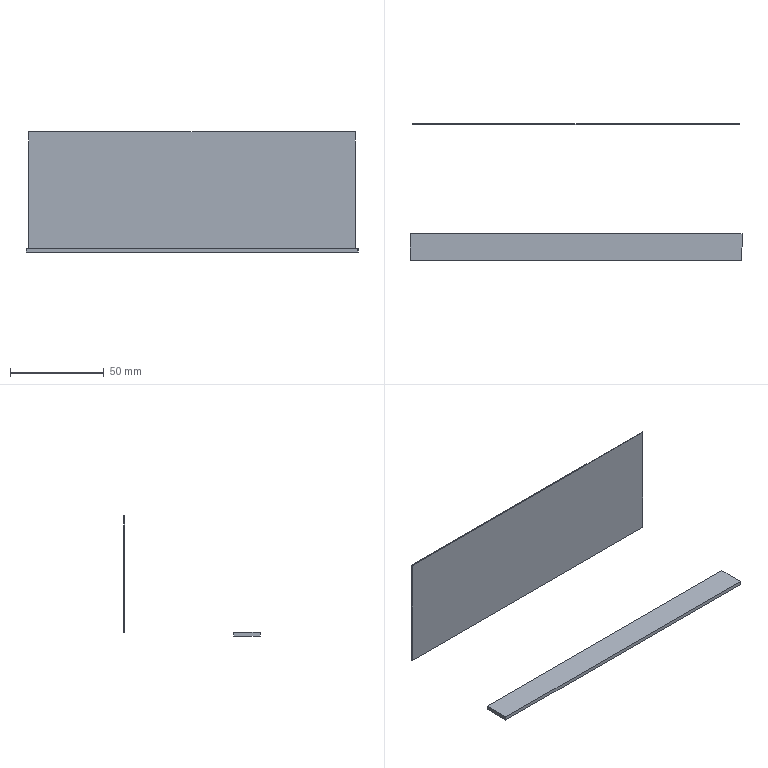Part | SolidWorks | features MirrorStock 1 | 2 solids | 12 faces | box 177 x 72.7 x 64 mm | volume 10414 mm3 | plane 12
STEP:
#1=CARTESIAN_POINT('',(-87.,30.,-62.));
#2=VERTEX_POINT('',#1);
#3=CARTESIAN_POINT('',(87.,30.,-62.));
#4=VERTEX_POINT('',#3);
#5=CARTESIAN_POINT('',(0.,30.,-62.));
#6=DIRECTION('',(1.,0.,0.));
#7=VECTOR('',#6,1000.);
#8=LINE('',#5,#7);
#9=EDGE_CURVE('',#2,#4,#8,.T.);
#10=ORIENTED_EDGE('',*,*,#9,.T.);
#11=CARTESIAN_POINT('',(87.,30.,0.));
#12=VERTEX_POINT('',#11);
#13=CARTESIAN_POINT('',(87.,30.,-31.));
#14=DIRECTION('',(0.,0.,1.));
#15=VECTOR('',#14,1000.);
#16=LINE('',#13,#15);
#17=EDGE_CURVE('',#4,#12,#16,.T.);
#18=ORIENTED_EDGE('',*,*,#17,.T.);
#19=CARTESIAN_POINT('',(-87.,30.,0.));
#20=VERTEX_POINT('',#19);
#21=CARTESIAN_POINT('',(0.,30.,0.));
#22=DIRECTION('',(-1.,0.,0.));
#23=VECTOR('',#22,1000.);
#24=LINE('',#21,#23);
#25=EDGE_CURVE('',#12,#20,#24,.T.);
#26=ORIENTED_EDGE('',*,*,#25,.T.);
#27=CARTESIAN_POINT('',(-87.,30.,-31.));
#28=DIRECTION('',(0.,0.,-1.));
#29=VECTOR('',#28,1000.);
#30=LINE('',#27,#29);
#31=EDGE_CURVE('',#20,#2,#30,.T.);
#32=ORIENTED_EDGE('',*,*,#31,.T.);
#33=EDGE_LOOP('',(#10,#18,#26,#32));
#34=FACE_OUTER_BOUND('',#33,.T.);
#35=CARTESIAN_POINT('',(90.48,30.,1.24));
#36=DIRECTION('',(0.,-1.,0.));
#37=DIRECTION('',(0.,0.,-1.));
#38=AXIS2_PLACEMENT_3D('',#35,#36,#37);
#39=PLANE('',#38);
#40=ADVANCED_FACE('',(#34),#39,.T.);
#41=ORIENTED_EDGE('',*,*,#25,.F.);
#42=CARTESIAN_POINT('',(87.,30.5,0.));
#43=VERTEX_POINT('',#42);
#44=CARTESIAN_POINT('',(87.,30.25,0.));
#45=DIRECTION('',(0.,1.,0.));
#46=VECTOR('',#45,1000.);
#47=LINE('',#44,#46);
#48=EDGE_CURVE('',#12,#43,#47,.T.);
#49=ORIENTED_EDGE('',*,*,#48,.T.);
#50=CARTESIAN_POINT('',(-87.,30.5,0.));
#51=VERTEX_POINT('',#50);
#52=CARTESIAN_POINT('',(0.,30.5,0.));
#53=DIRECTION('',(1.,0.,0.));
#54=VECTOR('',#53,1000.);
#55=LINE('',#52,#54);
#56=EDGE_CURVE('',#51,#43,#55,.T.);
#57=ORIENTED_EDGE('',*,*,#56,.F.);
#58=CARTESIAN_POINT('',(-87.,30.25,0.));
#59=DIRECTION('',(0.,-1.,0.));
#60=VECTOR('',#59,1000.);
#61=LINE('',#58,#60);
#62=EDGE_CURVE('',#51,#20,#61,.T.);
#63=ORIENTED_EDGE('',*,*,#62,.T.);
#64=EDGE_LOOP('',(#41,#49,#57,#63));
#65=FACE_OUTER_BOUND('',#64,.T.);
#66=CARTESIAN_POINT('',(-90.48,30.742,0.));
#67=DIRECTION('',(0.,0.,1.));
#68=DIRECTION('',(1.,0.,0.));
#69=AXIS2_PLACEMENT_3D('',#66,#67,#68);
#70=PLANE('',#69);
#71=ADVANCED_FACE('',(#65),#70,.T.);
#72=ORIENTED_EDGE('',*,*,#17,.F.);
#73=CARTESIAN_POINT('',(87.,30.5,-62.));
#74=VERTEX_POINT('',#73);
#75=CARTESIAN_POINT('',(87.,30.25,-62.));
#76=DIRECTION('',(0.,1.,0.));
#77=VECTOR('',#76,1000.);
#78=LINE('',#75,#77);
#79=EDGE_CURVE('',#4,#74,#78,.T.);
#80=ORIENTED_EDGE('',*,*,#79,.T.);
#81=CARTESIAN_POINT('',(87.,30.5,-31.));
#82=DIRECTION('',(0.,0.,-1.));
#83=VECTOR('',#82,1000.);
#84=LINE('',#81,#83);
#85=EDGE_CURVE('',#43,#74,#84,.T.);
#86=ORIENTED_EDGE('',*,*,#85,.F.);
#87=ORIENTED_EDGE('',*,*,#48,.F.);
#88=EDGE_LOOP('',(#72,#80,#86,#87));
#89=FACE_OUTER_BOUND('',#88,.T.);
#90=CARTESIAN_POINT('',(87.,30.742,1.24));
#91=DIRECTION('',(1.,0.,0.));
#92=DIRECTION('',(0.,0.,-1.));
#93=AXIS2_PLACEMENT_3D('',#90,#91,#92);
#94=PLANE('',#93);
#95=ADVANCED_FACE('',(#89),#94,.T.);
#96=ORIENTED_EDGE('',*,*,#9,.F.);
#97=CARTESIAN_POINT('',(-87.,30.5,-62.));
#98=VERTEX_POINT('',#97);
#99=CARTESIAN_POINT('',(-87.,30.25,-62.));
#100=DIRECTION('',(0.,1.,0.));
#101=VECTOR('',#100,1000.);
#102=LINE('',#99,#101);
#103=EDGE_CURVE('',#2,#98,#102,.T.);
#104=ORIENTED_EDGE('',*,*,#103,.T.);
#105=CARTESIAN_POINT('',(0.,30.5,-62.));
#106=DIRECTION('',(-1.,0.,0.));
#107=VECTOR('',#106,1000.);
#108=LINE('',#105,#107);
#109=EDGE_CURVE('',#74,#98,#108,.T.);
#110=ORIENTED_EDGE('',*,*,#109,.F.);
#111=ORIENTED_EDGE('',*,*,#79,.F.);
#112=EDGE_LOOP('',(#96,#104,#110,#111));
#113=FACE_OUTER_BOUND('',#112,.T.);
#114=CARTESIAN_POINT('',(90.48,30.742,-62.));
#115=DIRECTION('',(0.,0.,-1.));
#116=DIRECTION('',(-1.,0.,0.));
#117=AXIS2_PLACEMENT_3D('',#114,#115,#116);
#118=PLANE('',#117);
#119=ADVANCED_FACE('',(#113),#118,.T.);
#120=ORIENTED_EDGE('',*,*,#31,.F.);
#121=ORIENTED_EDGE('',*,*,#62,.F.);
#122=CARTESIAN_POINT('',(-87.,30.5,-31.));
#123=DIRECTION('',(0.,0.,1.));
#124=VECTOR('',#123,1000.);
#125=LINE('',#122,#124);
#126=EDGE_CURVE('',#98,#51,#125,.T.);
#127=ORIENTED_EDGE('',*,*,#126,.F.);
#128=ORIENTED_EDGE('',*,*,#103,.F.);
#129=EDGE_LOOP('',(#120,#121,#127,#128));
#130=FACE_OUTER_BOUND('',#129,.T.);
#131=CARTESIAN_POINT('',(-87.,30.742,-63.24));
#132=DIRECTION('',(-1.,0.,0.));
#133=DIRECTION('',(0.,0.,1.));
#134=AXIS2_PLACEMENT_3D('',#131,#132,#133);
#135=PLANE('',#134);
#136=ADVANCED_FACE('',(#130),#135,.T.);
#137=ORIENTED_EDGE('',*,*,#109,.T.);
#138=ORIENTED_EDGE('',*,*,#126,.T.);
#139=ORIENTED_EDGE('',*,*,#56,.T.);
#140=ORIENTED_EDGE('',*,*,#85,.T.);
#141=EDGE_LOOP('',(#137,#138,#139,#140));
#142=FACE_OUTER_BOUND('',#141,.T.);
#143=CARTESIAN_POINT('',(90.48,30.5,1.24));
#144=DIRECTION('',(0.,-1.,0.));
#145=DIRECTION('',(0.,0.,-1.));
#146=AXIS2_PLACEMENT_3D('',#143,#144,#145);
#147=PLANE('',#146);
#148=ADVANCED_FACE('',(#142),#147,.F.);
#149=CLOSED_SHELL('',(#40,#71,#95,#119,#136,#148));
#150=MANIFOLD_SOLID_BREP('',#149);
#151=CARTESIAN_POINT('',(-88.5,-42.2,-62.));
#152=VERTEX_POINT('',#151);
#153=CARTESIAN_POINT('',(88.5,-42.2,-62.));
#154=VERTEX_POINT('',#153);
#155=CARTESIAN_POINT('',(0.,-42.2,-62.));
#156=DIRECTION('',(1.,0.,0.));
#157=VECTOR('',#156,1000.);
#158=LINE('',#155,#157);
#159=EDGE_CURVE('',#152,#154,#158,.T.);
#160=ORIENTED_EDGE('',*,*,#159,.T.);
#161=CARTESIAN_POINT('',(88.5,-28.02,-62.));
#162=VERTEX_POINT('',#161);
#163=CARTESIAN_POINT('',(88.5,-35.11,-62.));
#164=DIRECTION('',(0.,1.,0.));
#165=VECTOR('',#164,1000.);
#166=LINE('',#163,#165);
#167=EDGE_CURVE('',#154,#162,#166,.T.);
#168=ORIENTED_EDGE('',*,*,#167,.T.);
#169=CARTESIAN_POINT('',(-88.5,-28.02,-62.));
#170=VERTEX_POINT('',#169);
#171=CARTESIAN_POINT('',(0.,-28.02,-62.));
#172=DIRECTION('',(-1.,0.,0.));
#173=VECTOR('',#172,1000.);
#174=LINE('',#171,#173);
#175=EDGE_CURVE('',#162,#170,#174,.T.);
#176=ORIENTED_EDGE('',*,*,#175,.T.);
#177=CARTESIAN_POINT('',(-88.5,-35.11,-62.));
#178=DIRECTION('',(0.,-1.,0.));
#179=VECTOR('',#178,1000.);
#180=LINE('',#177,#179);
#181=EDGE_CURVE('',#170,#152,#180,.T.);
#182=ORIENTED_EDGE('',*,*,#181,.T.);
#183=EDGE_LOOP('',(#160,#168,#176,#182));
#184=FACE_OUTER_BOUND('',#183,.T.);
#185=CARTESIAN_POINT('',(92.04,-27.737,-62.));
#186=DIRECTION('',(0.,0.,1.));
#187=DIRECTION('',(0.,-1.,0.));
#188=AXIS2_PLACEMENT_3D('',#185,#186,#187);
#189=PLANE('',#188);
#190=ADVANCED_FACE('',(#184),#189,.T.);
#191=ORIENTED_EDGE('',*,*,#175,.F.);
#192=CARTESIAN_POINT('',(88.5,-28.02,-64.));
#193=VERTEX_POINT('',#192);
#194=CARTESIAN_POINT('',(88.5,-28.02,-63.));
#195=DIRECTION('',(0.,0.,-1.));
#196=VECTOR('',#195,1000.);
#197=LINE('',#194,#196);
#198=EDGE_CURVE('',#162,#193,#197,.T.);
#199=ORIENTED_EDGE('',*,*,#198,.T.);
#200=CARTESIAN_POINT('',(-88.5,-28.02,-64.));
#201=VERTEX_POINT('',#200);
#202=CARTESIAN_POINT('',(0.,-28.02,-64.));
#203=DIRECTION('',(1.,0.,0.));
#204=VECTOR('',#203,1000.);
#205=LINE('',#202,#204);
#206=EDGE_CURVE('',#201,#193,#205,.T.);
#207=ORIENTED_EDGE('',*,*,#206,.F.);
#208=CARTESIAN_POINT('',(-88.5,-28.02,-63.));
#209=DIRECTION('',(0.,0.,1.));
#210=VECTOR('',#209,1000.);
#211=LINE('',#208,#210);
#212=EDGE_CURVE('',#201,#170,#211,.T.);
#213=ORIENTED_EDGE('',*,*,#212,.T.);
#214=EDGE_LOOP('',(#191,#199,#207,#213));
#215=FACE_OUTER_BOUND('',#214,.T.);
#216=CARTESIAN_POINT('',(-92.04,-28.02,-64.242));
#217=DIRECTION('',(0.,1.,0.));
#218=DIRECTION('',(1.,0.,0.));
#219=AXIS2_PLACEMENT_3D('',#216,#217,#218);
#220=PLANE('',#219);
#221=ADVANCED_FACE('',(#215),#220,.T.);
#222=ORIENTED_EDGE('',*,*,#167,.F.);
#223=CARTESIAN_POINT('',(88.5,-42.2,-64.));
#224=VERTEX_POINT('',#223);
#225=CARTESIAN_POINT('',(88.5,-42.2,-63.));
#226=DIRECTION('',(0.,0.,-1.));
#227=VECTOR('',#226,1000.);
#228=LINE('',#225,#227);
#229=EDGE_CURVE('',#154,#224,#228,.T.);
#230=ORIENTED_EDGE('',*,*,#229,.T.);
#231=CARTESIAN_POINT('',(88.5,-35.11,-64.));
#232=DIRECTION('',(0.,-1.,0.));
#233=VECTOR('',#232,1000.);
#234=LINE('',#231,#233);
#235=EDGE_CURVE('',#193,#224,#234,.T.);
#236=ORIENTED_EDGE('',*,*,#235,.F.);
#237=ORIENTED_EDGE('',*,*,#198,.F.);
#238=EDGE_LOOP('',(#222,#230,#236,#237));
#239=FACE_OUTER_BOUND('',#238,.T.);
#240=CARTESIAN_POINT('',(88.5,-27.737,-64.242));
#241=DIRECTION('',(1.,0.,0.));
#242=DIRECTION('',(0.,-1.,0.));
#243=AXIS2_PLACEMENT_3D('',#240,#241,#242);
#244=PLANE('',#243);
#245=ADVANCED_FACE('',(#239),#244,.T.);
#246=ORIENTED_EDGE('',*,*,#159,.F.);
#247=CARTESIAN_POINT('',(-88.5,-42.2,-64.));
#248=VERTEX_POINT('',#247);
#249=CARTESIAN_POINT('',(-88.5,-42.2,-63.));
#250=DIRECTION('',(0.,0.,-1.));
#251=VECTOR('',#250,1000.);
#252=LINE('',#249,#251);
#253=EDGE_CURVE('',#152,#248,#252,.T.);
#254=ORIENTED_EDGE('',*,*,#253,.T.);
#255=CARTESIAN_POINT('',(0.,-42.2,-64.));
#256=DIRECTION('',(-1.,0.,0.));
#257=VECTOR('',#256,1000.);
#258=LINE('',#255,#257);
#259=EDGE_CURVE('',#224,#248,#258,.T.);
#260=ORIENTED_EDGE('',*,*,#259,.F.);
#261=ORIENTED_EDGE('',*,*,#229,.F.);
#262=EDGE_LOOP('',(#246,#254,#260,#261));
#263=FACE_OUTER_BOUND('',#262,.T.);
#264=CARTESIAN_POINT('',(92.04,-42.2,-64.242));
#265=DIRECTION('',(0.,-1.,0.));
#266=DIRECTION('',(-1.,0.,0.));
#267=AXIS2_PLACEMENT_3D('',#264,#265,#266);
#268=PLANE('',#267);
#269=ADVANCED_FACE('',(#263),#268,.T.);
#270=ORIENTED_EDGE('',*,*,#181,.F.);
#271=ORIENTED_EDGE('',*,*,#212,.F.);
#272=CARTESIAN_POINT('',(-88.5,-35.11,-64.));
#273=DIRECTION('',(0.,1.,0.));
#274=VECTOR('',#273,1000.);
#275=LINE('',#272,#274);
#276=EDGE_CURVE('',#248,#201,#275,.T.);
#277=ORIENTED_EDGE('',*,*,#276,.F.);
#278=ORIENTED_EDGE('',*,*,#253,.F.);
#279=EDGE_LOOP('',(#270,#271,#277,#278));
#280=FACE_OUTER_BOUND('',#279,.T.);
#281=CARTESIAN_POINT('',(-88.5,-42.484,-64.242));
#282=DIRECTION('',(-1.,0.,0.));
#283=DIRECTION('',(0.,1.,0.));
#284=AXIS2_PLACEMENT_3D('',#281,#282,#283);
#285=PLANE('',#284);
#286=ADVANCED_FACE('',(#280),#285,.T.);
#287=ORIENTED_EDGE('',*,*,#259,.T.);
#288=ORIENTED_EDGE('',*,*,#276,.T.);
#289=ORIENTED_EDGE('',*,*,#206,.T.);
#290=ORIENTED_EDGE('',*,*,#235,.T.);
#291=EDGE_LOOP('',(#287,#288,#289,#290));
#292=FACE_OUTER_BOUND('',#291,.T.);
#293=CARTESIAN_POINT('',(92.04,-27.737,-64.));
#294=DIRECTION('',(0.,0.,1.));
#295=DIRECTION('',(0.,-1.,0.));
#296=AXIS2_PLACEMENT_3D('',#293,#294,#295);
#297=PLANE('',#296);
#298=ADVANCED_FACE('',(#292),#297,.F.);
#299=CLOSED_SHELL('',(#190,#221,#245,#269,#286,#298));
#300=MANIFOLD_SOLID_BREP('',#299);
#301=CARTESIAN_POINT('',(0.,0.,0.));
#302=DIRECTION('',(0.,0.,1.));
#303=DIRECTION('',(1.,0.,0.));
#304=AXIS2_PLACEMENT_3D('',#301,#302,#303);
#305=(LENGTH_UNIT()NAMED_UNIT(*)SI_UNIT(.MILLI.,.METRE.));
#306=UNCERTAINTY_MEASURE_WITH_UNIT(LENGTH_MEASURE(0.00001),#305,'','');
#307=(NAMED_UNIT(*)PLANE_ANGLE_UNIT()SI_UNIT($,.RADIAN.));
#308=(NAMED_UNIT(*)SI_UNIT($,.STERADIAN.)SOLID_ANGLE_UNIT());
#309=(GEOMETRIC_REPRESENTATION_CONTEXT(3)GLOBAL_UNCERTAINTY_ASSIGNED_CONTEXT((#306))GLOBAL_UNIT_ASSIGNED_CONTEXT((#305,#307,#308))REPRESENTATION_CONTEXT('',''));
#310=ADVANCED_BREP_SHAPE_REPRESENTATION('',(#150,#300,#304),#309);